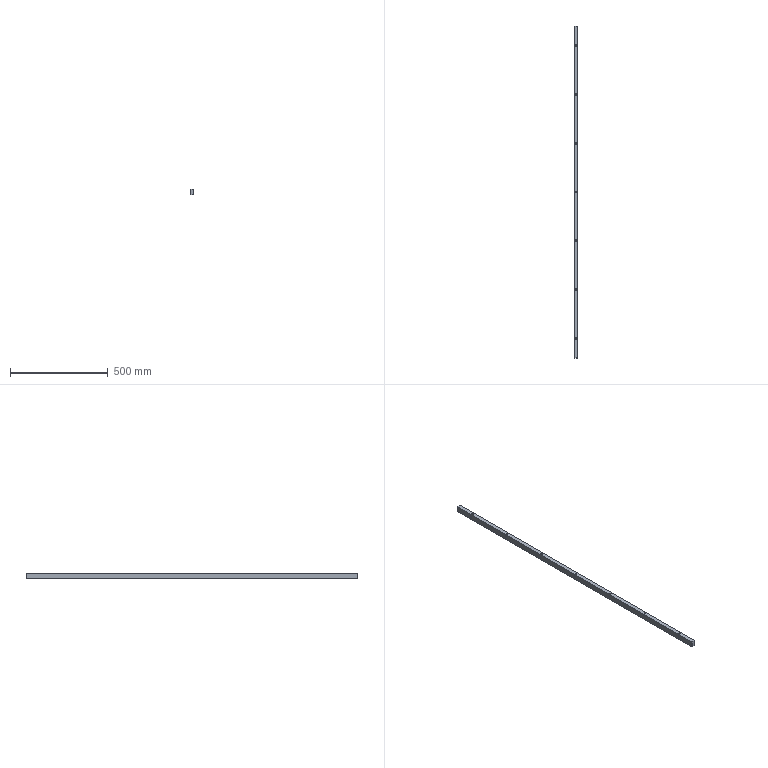Part | SolidWorks | features Chamfer 1, Extrusion 1, HoleWzd 1 | 1 solid | 45 faces | box 18 x 1700 x 30 mm | volume 889358 mm3 | cylinder 28 | plane 17 | commonest cylinder face diameters 9 x14 15 x14
STEP:
#1=CARTESIAN_POINT('',(16.5,1600.,-11.));
#2=VERTEX_POINT('',#1);
#3=CARTESIAN_POINT('',(1.5,1600.,-11.));
#4=VERTEX_POINT('',#3);
#5=CARTESIAN_POINT('',(9.,1600.,-11.));
#6=DIRECTION('',(0.,0.,-1.));
#7=DIRECTION('',(-1.,0.,0.));
#8=AXIS2_PLACEMENT_3D('',#5,#6,#7);
#9=CIRCLE('',#8,7.5);
#10=EDGE_CURVE('',#2,#4,#9,.T.);
#11=ORIENTED_EDGE('',*,*,#10,.F.);
#12=CARTESIAN_POINT('',(16.5,1600.,-30.));
#13=VERTEX_POINT('',#12);
#14=CARTESIAN_POINT('',(16.5,1600.,-30.));
#15=DIRECTION('',(0.,0.,-1.));
#16=VECTOR('',#15,1000.);
#17=LINE('',#14,#16);
#18=EDGE_CURVE('',#2,#13,#17,.T.);
#19=ORIENTED_EDGE('',*,*,#18,.T.);
#20=CARTESIAN_POINT('',(1.5,1600.,-30.));
#21=VERTEX_POINT('',#20);
#22=CARTESIAN_POINT('',(9.,1600.,-30.));
#23=DIRECTION('',(0.,0.,-1.));
#24=DIRECTION('',(-1.,0.,0.));
#25=AXIS2_PLACEMENT_3D('',#22,#23,#24);
#26=CIRCLE('',#25,7.5);
#27=EDGE_CURVE('',#13,#21,#26,.T.);
#28=ORIENTED_EDGE('',*,*,#27,.T.);
#29=CARTESIAN_POINT('',(1.5,1600.,-30.));
#30=DIRECTION('',(0.,0.,-1.));
#31=VECTOR('',#30,1000.);
#32=LINE('',#29,#31);
#33=EDGE_CURVE('',#4,#21,#32,.T.);
#34=ORIENTED_EDGE('',*,*,#33,.F.);
#35=EDGE_LOOP('',(#11,#19,#28,#34));
#36=FACE_OUTER_BOUND('',#35,.T.);
#37=CARTESIAN_POINT('',(9.,1600.,-30.));
#38=DIRECTION('',(0.,0.,-1.));
#39=DIRECTION('',(-1.,0.,0.));
#40=AXIS2_PLACEMENT_3D('',#37,#38,#39);
#41=CYLINDRICAL_SURFACE('',#40,7.5);
#42=ADVANCED_FACE('',(#36),#41,.F.);
#43=CARTESIAN_POINT('',(13.5,1600.,0.));
#44=VERTEX_POINT('',#43);
#45=CARTESIAN_POINT('',(4.5,1600.,0.));
#46=VERTEX_POINT('',#45);
#47=CARTESIAN_POINT('',(9.,1600.,0.));
#48=DIRECTION('',(0.,0.,-1.));
#49=DIRECTION('',(-1.,0.,0.));
#50=AXIS2_PLACEMENT_3D('',#47,#48,#49);
#51=CIRCLE('',#50,4.5);
#52=EDGE_CURVE('',#44,#46,#51,.T.);
#53=ORIENTED_EDGE('',*,*,#52,.F.);
#54=CARTESIAN_POINT('',(13.5,1600.,-11.));
#55=VERTEX_POINT('',#54);
#56=CARTESIAN_POINT('',(13.5,1600.,-30.));
#57=DIRECTION('',(0.,0.,-1.));
#58=VECTOR('',#57,1000.);
#59=LINE('',#56,#58);
#60=EDGE_CURVE('',#44,#55,#59,.T.);
#61=ORIENTED_EDGE('',*,*,#60,.T.);
#62=CARTESIAN_POINT('',(4.5,1600.,-11.));
#63=VERTEX_POINT('',#62);
#64=CARTESIAN_POINT('',(9.,1600.,-11.));
#65=DIRECTION('',(0.,0.,-1.));
#66=DIRECTION('',(-1.,0.,0.));
#67=AXIS2_PLACEMENT_3D('',#64,#65,#66);
#68=CIRCLE('',#67,4.5);
#69=EDGE_CURVE('',#55,#63,#68,.T.);
#70=ORIENTED_EDGE('',*,*,#69,.T.);
#71=CARTESIAN_POINT('',(4.5,1600.,-30.));
#72=DIRECTION('',(0.,0.,-1.));
#73=VECTOR('',#72,1000.);
#74=LINE('',#71,#73);
#75=EDGE_CURVE('',#46,#63,#74,.T.);
#76=ORIENTED_EDGE('',*,*,#75,.F.);
#77=EDGE_LOOP('',(#53,#61,#70,#76));
#78=FACE_OUTER_BOUND('',#77,.T.);
#79=CARTESIAN_POINT('',(9.,1600.,-30.));
#80=DIRECTION('',(0.,0.,-1.));
#81=DIRECTION('',(-1.,0.,0.));
#82=AXIS2_PLACEMENT_3D('',#79,#80,#81);
#83=CYLINDRICAL_SURFACE('',#82,4.5);
#84=ADVANCED_FACE('',(#78),#83,.F.);
#85=CARTESIAN_POINT('',(16.5,1350.,-11.));
#86=VERTEX_POINT('',#85);
#87=CARTESIAN_POINT('',(1.5,1350.,-11.));
#88=VERTEX_POINT('',#87);
#89=CARTESIAN_POINT('',(9.,1350.,-11.));
#90=DIRECTION('',(0.,0.,-1.));
#91=DIRECTION('',(-1.,0.,0.));
#92=AXIS2_PLACEMENT_3D('',#89,#90,#91);
#93=CIRCLE('',#92,7.5);
#94=EDGE_CURVE('',#86,#88,#93,.T.);
#95=ORIENTED_EDGE('',*,*,#94,.F.);
#96=CARTESIAN_POINT('',(16.5,1350.,-30.));
#97=VERTEX_POINT('',#96);
#98=CARTESIAN_POINT('',(16.5,1350.,-30.));
#99=DIRECTION('',(0.,0.,-1.));
#100=VECTOR('',#99,1000.);
#101=LINE('',#98,#100);
#102=EDGE_CURVE('',#86,#97,#101,.T.);
#103=ORIENTED_EDGE('',*,*,#102,.T.);
#104=CARTESIAN_POINT('',(1.5,1350.,-30.));
#105=VERTEX_POINT('',#104);
#106=CARTESIAN_POINT('',(9.,1350.,-30.));
#107=DIRECTION('',(0.,0.,-1.));
#108=DIRECTION('',(-1.,0.,0.));
#109=AXIS2_PLACEMENT_3D('',#106,#107,#108);
#110=CIRCLE('',#109,7.5);
#111=EDGE_CURVE('',#97,#105,#110,.T.);
#112=ORIENTED_EDGE('',*,*,#111,.T.);
#113=CARTESIAN_POINT('',(1.5,1350.,-30.));
#114=DIRECTION('',(0.,0.,-1.));
#115=VECTOR('',#114,1000.);
#116=LINE('',#113,#115);
#117=EDGE_CURVE('',#88,#105,#116,.T.);
#118=ORIENTED_EDGE('',*,*,#117,.F.);
#119=EDGE_LOOP('',(#95,#103,#112,#118));
#120=FACE_OUTER_BOUND('',#119,.T.);
#121=CARTESIAN_POINT('',(9.,1350.,-30.));
#122=DIRECTION('',(0.,0.,-1.));
#123=DIRECTION('',(-1.,0.,0.));
#124=AXIS2_PLACEMENT_3D('',#121,#122,#123);
#125=CYLINDRICAL_SURFACE('',#124,7.5);
#126=ADVANCED_FACE('',(#120),#125,.F.);
#127=CARTESIAN_POINT('',(13.5,1350.,0.));
#128=VERTEX_POINT('',#127);
#129=CARTESIAN_POINT('',(4.5,1350.,0.));
#130=VERTEX_POINT('',#129);
#131=CARTESIAN_POINT('',(9.,1350.,0.));
#132=DIRECTION('',(0.,0.,-1.));
#133=DIRECTION('',(-1.,0.,0.));
#134=AXIS2_PLACEMENT_3D('',#131,#132,#133);
#135=CIRCLE('',#134,4.5);
#136=EDGE_CURVE('',#128,#130,#135,.T.);
#137=ORIENTED_EDGE('',*,*,#136,.F.);
#138=CARTESIAN_POINT('',(13.5,1350.,-11.));
#139=VERTEX_POINT('',#138);
#140=CARTESIAN_POINT('',(13.5,1350.,-30.));
#141=DIRECTION('',(0.,0.,-1.));
#142=VECTOR('',#141,1000.);
#143=LINE('',#140,#142);
#144=EDGE_CURVE('',#128,#139,#143,.T.);
#145=ORIENTED_EDGE('',*,*,#144,.T.);
#146=CARTESIAN_POINT('',(4.5,1350.,-11.));
#147=VERTEX_POINT('',#146);
#148=CARTESIAN_POINT('',(9.,1350.,-11.));
#149=DIRECTION('',(0.,0.,-1.));
#150=DIRECTION('',(-1.,0.,0.));
#151=AXIS2_PLACEMENT_3D('',#148,#149,#150);
#152=CIRCLE('',#151,4.5);
#153=EDGE_CURVE('',#139,#147,#152,.T.);
#154=ORIENTED_EDGE('',*,*,#153,.T.);
#155=CARTESIAN_POINT('',(4.5,1350.,-30.));
#156=DIRECTION('',(0.,0.,-1.));
#157=VECTOR('',#156,1000.);
#158=LINE('',#155,#157);
#159=EDGE_CURVE('',#130,#147,#158,.T.);
#160=ORIENTED_EDGE('',*,*,#159,.F.);
#161=EDGE_LOOP('',(#137,#145,#154,#160));
#162=FACE_OUTER_BOUND('',#161,.T.);
#163=CARTESIAN_POINT('',(9.,1350.,-30.));
#164=DIRECTION('',(0.,0.,-1.));
#165=DIRECTION('',(-1.,0.,0.));
#166=AXIS2_PLACEMENT_3D('',#163,#164,#165);
#167=CYLINDRICAL_SURFACE('',#166,4.5);
#168=ADVANCED_FACE('',(#162),#167,.F.);
#169=CARTESIAN_POINT('',(16.5,1100.,-11.));
#170=VERTEX_POINT('',#169);
#171=CARTESIAN_POINT('',(1.5,1100.,-11.));
#172=VERTEX_POINT('',#171);
#173=CARTESIAN_POINT('',(9.,1100.,-11.));
#174=DIRECTION('',(0.,0.,-1.));
#175=DIRECTION('',(-1.,0.,0.));
#176=AXIS2_PLACEMENT_3D('',#173,#174,#175);
#177=CIRCLE('',#176,7.5);
#178=EDGE_CURVE('',#170,#172,#177,.T.);
#179=ORIENTED_EDGE('',*,*,#178,.F.);
#180=CARTESIAN_POINT('',(16.5,1100.,-30.));
#181=VERTEX_POINT('',#180);
#182=CARTESIAN_POINT('',(16.5,1100.,-30.));
#183=DIRECTION('',(0.,0.,-1.));
#184=VECTOR('',#183,1000.);
#185=LINE('',#182,#184);
#186=EDGE_CURVE('',#170,#181,#185,.T.);
#187=ORIENTED_EDGE('',*,*,#186,.T.);
#188=CARTESIAN_POINT('',(1.5,1100.,-30.));
#189=VERTEX_POINT('',#188);
#190=CARTESIAN_POINT('',(9.,1100.,-30.));
#191=DIRECTION('',(0.,0.,-1.));
#192=DIRECTION('',(-1.,0.,0.));
#193=AXIS2_PLACEMENT_3D('',#190,#191,#192);
#194=CIRCLE('',#193,7.5);
#195=EDGE_CURVE('',#181,#189,#194,.T.);
#196=ORIENTED_EDGE('',*,*,#195,.T.);
#197=CARTESIAN_POINT('',(1.5,1100.,-30.));
#198=DIRECTION('',(0.,0.,-1.));
#199=VECTOR('',#198,1000.);
#200=LINE('',#197,#199);
#201=EDGE_CURVE('',#172,#189,#200,.T.);
#202=ORIENTED_EDGE('',*,*,#201,.F.);
#203=EDGE_LOOP('',(#179,#187,#196,#202));
#204=FACE_OUTER_BOUND('',#203,.T.);
#205=CARTESIAN_POINT('',(9.,1100.,-30.));
#206=DIRECTION('',(0.,0.,-1.));
#207=DIRECTION('',(-1.,0.,0.));
#208=AXIS2_PLACEMENT_3D('',#205,#206,#207);
#209=CYLINDRICAL_SURFACE('',#208,7.5);
#210=ADVANCED_FACE('',(#204),#209,.F.);
#211=CARTESIAN_POINT('',(13.5,1100.,0.));
#212=VERTEX_POINT('',#211);
#213=CARTESIAN_POINT('',(4.5,1100.,0.));
#214=VERTEX_POINT('',#213);
#215=CARTESIAN_POINT('',(9.,1100.,0.));
#216=DIRECTION('',(0.,0.,-1.));
#217=DIRECTION('',(-1.,0.,0.));
#218=AXIS2_PLACEMENT_3D('',#215,#216,#217);
#219=CIRCLE('',#218,4.5);
#220=EDGE_CURVE('',#212,#214,#219,.T.);
#221=ORIENTED_EDGE('',*,*,#220,.F.);
#222=CARTESIAN_POINT('',(13.5,1100.,-11.));
#223=VERTEX_POINT('',#222);
#224=CARTESIAN_POINT('',(13.5,1100.,-30.));
#225=DIRECTION('',(0.,0.,-1.));
#226=VECTOR('',#225,1000.);
#227=LINE('',#224,#226);
#228=EDGE_CURVE('',#212,#223,#227,.T.);
#229=ORIENTED_EDGE('',*,*,#228,.T.);
#230=CARTESIAN_POINT('',(4.5,1100.,-11.));
#231=VERTEX_POINT('',#230);
#232=CARTESIAN_POINT('',(9.,1100.,-11.));
#233=DIRECTION('',(0.,0.,-1.));
#234=DIRECTION('',(-1.,0.,0.));
#235=AXIS2_PLACEMENT_3D('',#232,#233,#234);
#236=CIRCLE('',#235,4.5);
#237=EDGE_CURVE('',#223,#231,#236,.T.);
#238=ORIENTED_EDGE('',*,*,#237,.T.);
#239=CARTESIAN_POINT('',(4.5,1100.,-30.));
#240=DIRECTION('',(0.,0.,-1.));
#241=VECTOR('',#240,1000.);
#242=LINE('',#239,#241);
#243=EDGE_CURVE('',#214,#231,#242,.T.);
#244=ORIENTED_EDGE('',*,*,#243,.F.);
#245=EDGE_LOOP('',(#221,#229,#238,#244));
#246=FACE_OUTER_BOUND('',#245,.T.);
#247=CARTESIAN_POINT('',(9.,1100.,-30.));
#248=DIRECTION('',(0.,0.,-1.));
#249=DIRECTION('',(-1.,0.,0.));
#250=AXIS2_PLACEMENT_3D('',#247,#248,#249);
#251=CYLINDRICAL_SURFACE('',#250,4.5);
#252=ADVANCED_FACE('',(#246),#251,.F.);
#253=CARTESIAN_POINT('',(16.5,600.,-11.));
#254=VERTEX_POINT('',#253);
#255=CARTESIAN_POINT('',(1.5,600.,-11.));
#256=VERTEX_POINT('',#255);
#257=CARTESIAN_POINT('',(9.,600.,-11.));
#258=DIRECTION('',(0.,0.,-1.));
#259=DIRECTION('',(-1.,0.,0.));
#260=AXIS2_PLACEMENT_3D('',#257,#258,#259);
#261=CIRCLE('',#260,7.5);
#262=EDGE_CURVE('',#254,#256,#261,.T.);
#263=ORIENTED_EDGE('',*,*,#262,.F.);
#264=CARTESIAN_POINT('',(16.5,600.,-30.));
#265=VERTEX_POINT('',#264);
#266=CARTESIAN_POINT('',(16.5,600.,-30.));
#267=DIRECTION('',(0.,0.,-1.));
#268=VECTOR('',#267,1000.);
#269=LINE('',#266,#268);
#270=EDGE_CURVE('',#254,#265,#269,.T.);
#271=ORIENTED_EDGE('',*,*,#270,.T.);
#272=CARTESIAN_POINT('',(1.5,600.,-30.));
#273=VERTEX_POINT('',#272);
#274=CARTESIAN_POINT('',(9.,600.,-30.));
#275=DIRECTION('',(0.,0.,-1.));
#276=DIRECTION('',(-1.,0.,0.));
#277=AXIS2_PLACEMENT_3D('',#274,#275,#276);
#278=CIRCLE('',#277,7.5);
#279=EDGE_CURVE('',#265,#273,#278,.T.);
#280=ORIENTED_EDGE('',*,*,#279,.T.);
#281=CARTESIAN_POINT('',(1.5,600.,-30.));
#282=DIRECTION('',(0.,0.,-1.));
#283=VECTOR('',#282,1000.);
#284=LINE('',#281,#283);
#285=EDGE_CURVE('',#256,#273,#284,.T.);
#286=ORIENTED_EDGE('',*,*,#285,.F.);
#287=EDGE_LOOP('',(#263,#271,#280,#286));
#288=FACE_OUTER_BOUND('',#287,.T.);
#289=CARTESIAN_POINT('',(9.,600.,-30.));
#290=DIRECTION('',(0.,0.,-1.));
#291=DIRECTION('',(-1.,0.,0.));
#292=AXIS2_PLACEMENT_3D('',#289,#290,#291);
#293=CYLINDRICAL_SURFACE('',#292,7.5);
#294=ADVANCED_FACE('',(#288),#293,.F.);
#295=CARTESIAN_POINT('',(13.5,600.,0.));
#296=VERTEX_POINT('',#295);
#297=CARTESIAN_POINT('',(4.5,600.,0.));
#298=VERTEX_POINT('',#297);
#299=CARTESIAN_POINT('',(9.,600.,0.));
#300=DIRECTION('',(0.,0.,-1.));
#301=DIRECTION('',(-1.,0.,0.));
#302=AXIS2_PLACEMENT_3D('',#299,#300,#301);
#303=CIRCLE('',#302,4.5);
#304=EDGE_CURVE('',#296,#298,#303,.T.);
#305=ORIENTED_EDGE('',*,*,#304,.F.);
#306=CARTESIAN_POINT('',(13.5,600.,-11.));
#307=VERTEX_POINT('',#306);
#308=CARTESIAN_POINT('',(13.5,600.,-30.));
#309=DIRECTION('',(0.,0.,-1.));
#310=VECTOR('',#309,1000.);
#311=LINE('',#308,#310);
#312=EDGE_CURVE('',#296,#307,#311,.T.);
#313=ORIENTED_EDGE('',*,*,#312,.T.);
#314=CARTESIAN_POINT('',(4.5,600.,-11.));
#315=VERTEX_POINT('',#314);
#316=CARTESIAN_POINT('',(9.,600.,-11.));
#317=DIRECTION('',(0.,0.,-1.));
#318=DIRECTION('',(-1.,0.,0.));
#319=AXIS2_PLACEMENT_3D('',#316,#317,#318);
#320=CIRCLE('',#319,4.5);
#321=EDGE_CURVE('',#307,#315,#320,.T.);
#322=ORIENTED_EDGE('',*,*,#321,.T.);
#323=CARTESIAN_POINT('',(4.5,600.,-30.));
#324=DIRECTION('',(0.,0.,-1.));
#325=VECTOR('',#324,1000.);
#326=LINE('',#323,#325);
#327=EDGE_CURVE('',#298,#315,#326,.T.);
#328=ORIENTED_EDGE('',*,*,#327,.F.);
#329=EDGE_LOOP('',(#305,#313,#322,#328));
#330=FACE_OUTER_BOUND('',#329,.T.);
#331=CARTESIAN_POINT('',(9.,600.,-30.));
#332=DIRECTION('',(0.,0.,-1.));
#333=DIRECTION('',(-1.,0.,0.));
#334=AXIS2_PLACEMENT_3D('',#331,#332,#333);
#335=CYLINDRICAL_SURFACE('',#334,4.5);
#336=ADVANCED_FACE('',(#330),#335,.F.);
#337=CARTESIAN_POINT('',(16.5,350.,-11.));
#338=VERTEX_POINT('',#337);
#339=CARTESIAN_POINT('',(1.5,350.,-11.));
#340=VERTEX_POINT('',#339);
#341=CARTESIAN_POINT('',(9.,350.,-11.));
#342=DIRECTION('',(0.,0.,-1.));
#343=DIRECTION('',(-1.,0.,0.));
#344=AXIS2_PLACEMENT_3D('',#341,#342,#343);
#345=CIRCLE('',#344,7.5);
#346=EDGE_CURVE('',#338,#340,#345,.T.);
#347=ORIENTED_EDGE('',*,*,#346,.F.);
#348=CARTESIAN_POINT('',(16.5,350.,-30.));
#349=VERTEX_POINT('',#348);
#350=CARTESIAN_POINT('',(16.5,350.,-30.));
#351=DIRECTION('',(0.,0.,-1.));
#352=VECTOR('',#351,1000.);
#353=LINE('',#350,#352);
#354=EDGE_CURVE('',#338,#349,#353,.T.);
#355=ORIENTED_EDGE('',*,*,#354,.T.);
#356=CARTESIAN_POINT('',(1.5,350.,-30.));
#357=VERTEX_POINT('',#356);
#358=CARTESIAN_POINT('',(9.,350.,-30.));
#359=DIRECTION('',(0.,0.,-1.));
#360=DIRECTION('',(-1.,0.,0.));
#361=AXIS2_PLACEMENT_3D('',#358,#359,#360);
#362=CIRCLE('',#361,7.5);
#363=EDGE_CURVE('',#349,#357,#362,.T.);
#364=ORIENTED_EDGE('',*,*,#363,.T.);
#365=CARTESIAN_POINT('',(1.5,350.,-30.));
#366=DIRECTION('',(0.,0.,-1.));
#367=VECTOR('',#366,1000.);
#368=LINE('',#365,#367);
#369=EDGE_CURVE('',#340,#357,#368,.T.);
#370=ORIENTED_EDGE('',*,*,#369,.F.);
#371=EDGE_LOOP('',(#347,#355,#364,#370));
#372=FACE_OUTER_BOUND('',#371,.T.);
#373=CARTESIAN_POINT('',(9.,350.,-30.));
#374=DIRECTION('',(0.,0.,-1.));
#375=DIRECTION('',(-1.,0.,0.));
#376=AXIS2_PLACEMENT_3D('',#373,#374,#375);
#377=CYLINDRICAL_SURFACE('',#376,7.5);
#378=ADVANCED_FACE('',(#372),#377,.F.);
#379=CARTESIAN_POINT('',(13.5,350.,0.));
#380=VERTEX_POINT('',#379);
#381=CARTESIAN_POINT('',(4.5,350.,0.));
#382=VERTEX_POINT('',#381);
#383=CARTESIAN_POINT('',(9.,350.,0.));
#384=DIRECTION('',(0.,0.,-1.));
#385=DIRECTION('',(-1.,0.,0.));
#386=AXIS2_PLACEMENT_3D('',#383,#384,#385);
#387=CIRCLE('',#386,4.5);
#388=EDGE_CURVE('',#380,#382,#387,.T.);
#389=ORIENTED_EDGE('',*,*,#388,.F.);
#390=CARTESIAN_POINT('',(13.5,350.,-11.));
#391=VERTEX_POINT('',#390);
#392=CARTESIAN_POINT('',(13.5,350.,-30.));
#393=DIRECTION('',(0.,0.,-1.));
#394=VECTOR('',#393,1000.);
#395=LINE('',#392,#394);
#396=EDGE_CURVE('',#380,#391,#395,.T.);
#397=ORIENTED_EDGE('',*,*,#396,.T.);
#398=CARTESIAN_POINT('',(4.5,350.,-11.));
#399=VERTEX_POINT('',#398);
#400=CARTESIAN_POINT('',(9.,350.,-11.));
#401=DIRECTION('',(0.,0.,-1.));
#402=DIRECTION('',(-1.,0.,0.));
#403=AXIS2_PLACEMENT_3D('',#400,#401,#402);
#404=CIRCLE('',#403,4.5);
#405=EDGE_CURVE('',#391,#399,#404,.T.);
#406=ORIENTED_EDGE('',*,*,#405,.T.);
#407=CARTESIAN_POINT('',(4.5,350.,-30.));
#408=DIRECTION('',(0.,0.,-1.));
#409=VECTOR('',#408,1000.);
#410=LINE('',#407,#409);
#411=EDGE_CURVE('',#382,#399,#410,.T.);
#412=ORIENTED_EDGE('',*,*,#411,.F.);
#413=EDGE_LOOP('',(#389,#397,#406,#412));
#414=FACE_OUTER_BOUND('',#413,.T.);
#415=CARTESIAN_POINT('',(9.,350.,-30.));
#416=DIRECTION('',(0.,0.,-1.));
#417=DIRECTION('',(-1.,0.,0.));
#418=AXIS2_PLACEMENT_3D('',#415,#416,#417);
#419=CYLINDRICAL_SURFACE('',#418,4.5);
#420=ADVANCED_FACE('',(#414),#419,.F.);
#421=CARTESIAN_POINT('',(16.5,100.,-11.));
#422=VERTEX_POINT('',#421);
#423=CARTESIAN_POINT('',(1.5,100.,-11.));
#424=VERTEX_POINT('',#423);
#425=CARTESIAN_POINT('',(9.,100.,-11.));
#426=DIRECTION('',(0.,0.,-1.));
#427=DIRECTION('',(-1.,0.,0.));
#428=AXIS2_PLACEMENT_3D('',#425,#426,#427);
#429=CIRCLE('',#428,7.5);
#430=EDGE_CURVE('',#422,#424,#429,.T.);
#431=ORIENTED_EDGE('',*,*,#430,.F.);
#432=CARTESIAN_POINT('',(16.5,100.,-30.));
#433=VERTEX_POINT('',#432);
#434=CARTESIAN_POINT('',(16.5,100.,-30.));
#435=DIRECTION('',(0.,0.,-1.));
#436=VECTOR('',#435,1000.);
#437=LINE('',#434,#436);
#438=EDGE_CURVE('',#422,#433,#437,.T.);
#439=ORIENTED_EDGE('',*,*,#438,.T.);
#440=CARTESIAN_POINT('',(1.5,100.,-30.));
#441=VERTEX_POINT('',#440);
#442=CARTESIAN_POINT('',(9.,100.,-30.));
#443=DIRECTION('',(0.,0.,-1.));
#444=DIRECTION('',(-1.,0.,0.));
#445=AXIS2_PLACEMENT_3D('',#442,#443,#444);
#446=CIRCLE('',#445,7.5);
#447=EDGE_CURVE('',#433,#441,#446,.T.);
#448=ORIENTED_EDGE('',*,*,#447,.T.);
#449=CARTESIAN_POINT('',(1.5,100.,-30.));
#450=DIRECTION('',(0.,0.,-1.));
#451=VECTOR('',#450,1000.);
#452=LINE('',#449,#451);
#453=EDGE_CURVE('',#424,#441,#452,.T.);
#454=ORIENTED_EDGE('',*,*,#453,.F.);
#455=EDGE_LOOP('',(#431,#439,#448,#454));
#456=FACE_OUTER_BOUND('',#455,.T.);
#457=CARTESIAN_POINT('',(9.,100.,-30.));
#458=DIRECTION('',(0.,0.,-1.));
#459=DIRECTION('',(-1.,0.,0.));
#460=AXIS2_PLACEMENT_3D('',#457,#458,#459);
#461=CYLINDRICAL_SURFACE('',#460,7.5);
#462=ADVANCED_FACE('',(#456),#461,.F.);
#463=CARTESIAN_POINT('',(13.5,100.,0.));
#464=VERTEX_POINT('',#463);
#465=CARTESIAN_POINT('',(4.5,100.,0.));
#466=VERTEX_POINT('',#465);
#467=CARTESIAN_POINT('',(9.,100.,0.));
#468=DIRECTION('',(0.,0.,-1.));
#469=DIRECTION('',(-1.,0.,0.));
#470=AXIS2_PLACEMENT_3D('',#467,#468,#469);
#471=CIRCLE('',#470,4.5);
#472=EDGE_CURVE('',#464,#466,#471,.T.);
#473=ORIENTED_EDGE('',*,*,#472,.F.);
#474=CARTESIAN_POINT('',(13.5,100.,-11.));
#475=VERTEX_POINT('',#474);
#476=CARTESIAN_POINT('',(13.5,100.,-30.));
#477=DIRECTION('',(0.,0.,-1.));
#478=VECTOR('',#477,1000.);
#479=LINE('',#476,#478);
#480=EDGE_CURVE('',#464,#475,#479,.T.);
#481=ORIENTED_EDGE('',*,*,#480,.T.);
#482=CARTESIAN_POINT('',(4.5,100.,-11.));
#483=VERTEX_POINT('',#482);
#484=CARTESIAN_POINT('',(9.,100.,-11.));
#485=DIRECTION('',(0.,0.,-1.));
#486=DIRECTION('',(-1.,0.,0.));
#487=AXIS2_PLACEMENT_3D('',#484,#485,#486);
#488=CIRCLE('',#487,4.5);
#489=EDGE_CURVE('',#475,#483,#488,.T.);
#490=ORIENTED_EDGE('',*,*,#489,.T.);
#491=CARTESIAN_POINT('',(4.5,100.,-30.));
#492=DIRECTION('',(0.,0.,-1.));
#493=VECTOR('',#492,1000.);
#494=LINE('',#491,#493);
#495=EDGE_CURVE('',#466,#483,#494,.T.);
#496=ORIENTED_EDGE('',*,*,#495,.F.);
#497=EDGE_LOOP('',(#473,#481,#490,#496));
#498=FACE_OUTER_BOUND('',#497,.T.);
#499=CARTESIAN_POINT('',(9.,100.,-30.));
#500=DIRECTION('',(0.,0.,-1.));
#501=DIRECTION('',(-1.,0.,0.));
#502=AXIS2_PLACEMENT_3D('',#499,#500,#501);
#503=CYLINDRICAL_SURFACE('',#502,4.5);
#504=ADVANCED_FACE('',(#498),#503,.F.);
#505=CARTESIAN_POINT('',(16.5,850.,-11.));
#506=VERTEX_POINT('',#505);
#507=CARTESIAN_POINT('',(1.5,850.,-11.));
#508=VERTEX_POINT('',#507);
#509=CARTESIAN_POINT('',(9.,850.,-11.));
#510=DIRECTION('',(0.,0.,-1.));
#511=DIRECTION('',(-1.,0.,0.));
#512=AXIS2_PLACEMENT_3D('',#509,#510,#511);
#513=CIRCLE('',#512,7.5);
#514=EDGE_CURVE('',#506,#508,#513,.T.);
#515=ORIENTED_EDGE('',*,*,#514,.F.);
#516=CARTESIAN_POINT('',(16.5,850.,-30.));
#517=VERTEX_POINT('',#516);
#518=CARTESIAN_POINT('',(16.5,850.,-30.));
#519=DIRECTION('',(0.,0.,-1.));
#520=VECTOR('',#519,1000.);
#521=LINE('',#518,#520);
#522=EDGE_CURVE('',#506,#517,#521,.T.);
#523=ORIENTED_EDGE('',*,*,#522,.T.);
#524=CARTESIAN_POINT('',(1.5,850.,-30.));
#525=VERTEX_POINT('',#524);
#526=CARTESIAN_POINT('',(9.,850.,-30.));
#527=DIRECTION('',(0.,0.,-1.));
#528=DIRECTION('',(-1.,0.,0.));
#529=AXIS2_PLACEMENT_3D('',#526,#527,#528);
#530=CIRCLE('',#529,7.5);
#531=EDGE_CURVE('',#517,#525,#530,.T.);
#532=ORIENTED_EDGE('',*,*,#531,.T.);
#533=CARTESIAN_POINT('',(1.5,850.,-30.));
#534=DIRECTION('',(0.,0.,-1.));
#535=VECTOR('',#534,1000.);
#536=LINE('',#533,#535);
#537=EDGE_CURVE('',#508,#525,#536,.T.);
#538=ORIENTED_EDGE('',*,*,#537,.F.);
#539=EDGE_LOOP('',(#515,#523,#532,#538));
#540=FACE_OUTER_BOUND('',#539,.T.);
#541=CARTESIAN_POINT('',(9.,850.,-30.));
#542=DIRECTION('',(0.,0.,-1.));
#543=DIRECTION('',(-1.,0.,0.));
#544=AXIS2_PLACEMENT_3D('',#541,#542,#543);
#545=CYLINDRICAL_SURFACE('',#544,7.5);
#546=ADVANCED_FACE('',(#540),#545,.F.);
#547=CARTESIAN_POINT('',(13.5,850.,0.));
#548=VERTEX_POINT('',#547);
#549=CARTESIAN_POINT('',(4.5,850.,0.));
#550=VERTEX_POINT('',#549);
#551=CARTESIAN_POINT('',(9.,850.,0.));
#552=DIRECTION('',(0.,0.,-1.));
#553=DIRECTION('',(-1.,0.,0.));
#554=AXIS2_PLACEMENT_3D('',#551,#552,#553);
#555=CIRCLE('',#554,4.5);
#556=EDGE_CURVE('',#548,#550,#555,.T.);
#557=ORIENTED_EDGE('',*,*,#556,.F.);
#558=CARTESIAN_POINT('',(13.5,850.,-11.));
#559=VERTEX_POINT('',#558);
#560=CARTESIAN_POINT('',(13.5,850.,-30.));
#561=DIRECTION('',(0.,0.,-1.));
#562=VECTOR('',#561,1000.);
#563=LINE('',#560,#562);
#564=EDGE_CURVE('',#548,#559,#563,.T.);
#565=ORIENTED_EDGE('',*,*,#564,.T.);
#566=CARTESIAN_POINT('',(4.5,850.,-11.));
#567=VERTEX_POINT('',#566);
#568=CARTESIAN_POINT('',(9.,850.,-11.));
#569=DIRECTION('',(0.,0.,-1.));
#570=DIRECTION('',(-1.,0.,0.));
#571=AXIS2_PLACEMENT_3D('',#568,#569,#570);
#572=CIRCLE('',#571,4.5);
#573=EDGE_CURVE('',#559,#567,#572,.T.);
#574=ORIENTED_EDGE('',*,*,#573,.T.);
#575=CARTESIAN_POINT('',(4.5,850.,-30.));
#576=DIRECTION('',(0.,0.,-1.));
#577=VECTOR('',#576,1000.);
#578=LINE('',#575,#577);
#579=EDGE_CURVE('',#550,#567,#578,.T.);
#580=ORIENTED_EDGE('',*,*,#579,.F.);
#581=EDGE_LOOP('',(#557,#565,#574,#580));
#582=FACE_OUTER_BOUND('',#581,.T.);
#583=CARTESIAN_POINT('',(9.,850.,-30.));
#584=DIRECTION('',(0.,0.,-1.));
#585=DIRECTION('',(-1.,0.,0.));
#586=AXIS2_PLACEMENT_3D('',#583,#584,#585);
#587=CYLINDRICAL_SURFACE('',#586,4.5);
#588=ADVANCED_FACE('',(#582),#587,.F.);
#589=CARTESIAN_POINT('',(9.,1600.,-30.));
#590=DIRECTION('',(0.,0.,-1.));
#591=DIRECTION('',(-1.,0.,0.));
#592=AXIS2_PLACEMENT_3D('',#589,#590,#591);
#593=CIRCLE('',#592,7.5);
#594=EDGE_CURVE('',#21,#13,#593,.T.);
#595=ORIENTED_EDGE('',*,*,#594,.F.);
#596=ORIENTED_EDGE('',*,*,#27,.F.);
#597=EDGE_LOOP('',(#595,#596));
#598=FACE_BOUND('',#597,.T.);
#599=CARTESIAN_POINT('',(9.,600.,-30.));
#600=DIRECTION('',(0.,0.,-1.));
#601=DIRECTION('',(-1.,0.,0.));
#602=AXIS2_PLACEMENT_3D('',#599,#600,#601);
#603=CIRCLE('',#602,7.5);
#604=EDGE_CURVE('',#273,#265,#603,.T.);
#605=ORIENTED_EDGE('',*,*,#604,.F.);
#606=ORIENTED_EDGE('',*,*,#279,.F.);
#607=EDGE_LOOP('',(#605,#606));
#608=FACE_BOUND('',#607,.T.);
#609=CARTESIAN_POINT('',(9.,100.,-30.));
#610=DIRECTION('',(0.,0.,-1.));
#611=DIRECTION('',(-1.,0.,0.));
#612=AXIS2_PLACEMENT_3D('',#609,#610,#611);
#613=CIRCLE('',#612,7.5);
#614=EDGE_CURVE('',#441,#433,#613,.T.);
#615=ORIENTED_EDGE('',*,*,#614,.F.);
#616=ORIENTED_EDGE('',*,*,#447,.F.);
#617=EDGE_LOOP('',(#615,#616));
#618=FACE_BOUND('',#617,.T.);
#619=CARTESIAN_POINT('',(9.,850.,-30.));
#620=DIRECTION('',(0.,0.,-1.));
#621=DIRECTION('',(-1.,0.,0.));
#622=AXIS2_PLACEMENT_3D('',#619,#620,#621);
#623=CIRCLE('',#622,7.5);
#624=EDGE_CURVE('',#525,#517,#623,.T.);
#625=ORIENTED_EDGE('',*,*,#624,.F.);
#626=ORIENTED_EDGE('',*,*,#531,.F.);
#627=EDGE_LOOP('',(#625,#626));
#628=FACE_BOUND('',#627,.T.);
#629=CARTESIAN_POINT('',(16.,0.,-30.));
#630=VERTEX_POINT('',#629);
#631=CARTESIAN_POINT('',(2.,0.,-30.));
#632=VERTEX_POINT('',#631);
#633=CARTESIAN_POINT('',(0.,0.,-30.));
#634=DIRECTION('',(-1.,0.,0.));
#635=VECTOR('',#634,1000.);
#636=LINE('',#633,#635);
#637=EDGE_CURVE('',#630,#632,#636,.T.);
#638=ORIENTED_EDGE('',*,*,#637,.T.);
#639=CARTESIAN_POINT('',(0.,2.,-30.));
#640=VERTEX_POINT('',#639);
#641=CARTESIAN_POINT('',(0.,2.,-30.));
#642=DIRECTION('',(-0.7071,0.7071,0.));
#643=VECTOR('',#642,1000.);
#644=LINE('',#641,#643);
#645=EDGE_CURVE('',#632,#640,#644,.T.);
#646=ORIENTED_EDGE('',*,*,#645,.T.);
#647=CARTESIAN_POINT('',(0.,1698.,-30.));
#648=VERTEX_POINT('',#647);
#649=CARTESIAN_POINT('',(0.,1700.,-30.));
#650=DIRECTION('',(0.,-1.,0.));
#651=VECTOR('',#650,1000.);
#652=LINE('',#649,#651);
#653=EDGE_CURVE('',#648,#640,#652,.T.);
#654=ORIENTED_EDGE('',*,*,#653,.F.);
#655=CARTESIAN_POINT('',(2.,1700.,-30.));
#656=VERTEX_POINT('',#655);
#657=CARTESIAN_POINT('',(2.,1700.,-30.));
#658=DIRECTION('',(0.7071,0.7071,0.));
#659=VECTOR('',#658,1000.);
#660=LINE('',#657,#659);
#661=EDGE_CURVE('',#648,#656,#660,.T.);
#662=ORIENTED_EDGE('',*,*,#661,.T.);
#663=CARTESIAN_POINT('',(16.,1700.,-30.));
#664=VERTEX_POINT('',#663);
#665=CARTESIAN_POINT('',(0.,1700.,-30.));
#666=DIRECTION('',(-1.,0.,0.));
#667=VECTOR('',#666,1000.);
#668=LINE('',#665,#667);
#669=EDGE_CURVE('',#664,#656,#668,.T.);
#670=ORIENTED_EDGE('',*,*,#669,.F.);
#671=CARTESIAN_POINT('',(18.,1698.,-30.));
#672=VERTEX_POINT('',#671);
#673=CARTESIAN_POINT('',(16.,1700.,-30.));
#674=DIRECTION('',(0.7071,-0.7071,0.));
#675=VECTOR('',#674,1000.);
#676=LINE('',#673,#675);
#677=EDGE_CURVE('',#664,#672,#676,.T.);
#678=ORIENTED_EDGE('',*,*,#677,.T.);
#679=CARTESIAN_POINT('',(18.,2.,-30.));
#680=VERTEX_POINT('',#679);
#681=CARTESIAN_POINT('',(18.,1700.,-30.));
#682=DIRECTION('',(0.,-1.,0.));
#683=VECTOR('',#682,1000.);
#684=LINE('',#681,#683);
#685=EDGE_CURVE('',#672,#680,#684,.T.);
#686=ORIENTED_EDGE('',*,*,#685,.T.);
#687=CARTESIAN_POINT('',(18.,2.,-30.));
#688=DIRECTION('',(-0.7071,-0.7071,0.));
#689=VECTOR('',#688,1000.);
#690=LINE('',#687,#689);
#691=EDGE_CURVE('',#680,#630,#690,.T.);
#692=ORIENTED_EDGE('',*,*,#691,.T.);
#693=EDGE_LOOP('',(#638,#646,#654,#662,#670,#678,#686,#692));
#694=FACE_OUTER_BOUND('',#693,.T.);
#695=CARTESIAN_POINT('',(9.,350.,-30.));
#696=DIRECTION('',(0.,0.,-1.));
#697=DIRECTION('',(-1.,0.,0.));
#698=AXIS2_PLACEMENT_3D('',#695,#696,#697);
#699=CIRCLE('',#698,7.5);
#700=EDGE_CURVE('',#357,#349,#699,.T.);
#701=ORIENTED_EDGE('',*,*,#700,.F.);
#702=ORIENTED_EDGE('',*,*,#363,.F.);
#703=EDGE_LOOP('',(#701,#702));
#704=FACE_BOUND('',#703,.T.);
#705=CARTESIAN_POINT('',(9.,1100.,-30.));
#706=DIRECTION('',(0.,0.,-1.));
#707=DIRECTION('',(-1.,0.,0.));
#708=AXIS2_PLACEMENT_3D('',#705,#706,#707);
#709=CIRCLE('',#708,7.5);
#710=EDGE_CURVE('',#189,#181,#709,.T.);
#711=ORIENTED_EDGE('',*,*,#710,.F.);
#712=ORIENTED_EDGE('',*,*,#195,.F.);
#713=EDGE_LOOP('',(#711,#712));
#714=FACE_BOUND('',#713,.T.);
#715=CARTESIAN_POINT('',(9.,1350.,-30.));
#716=DIRECTION('',(0.,0.,-1.));
#717=DIRECTION('',(-1.,0.,0.));
#718=AXIS2_PLACEMENT_3D('',#715,#716,#717);
#719=CIRCLE('',#718,7.5);
#720=EDGE_CURVE('',#105,#97,#719,.T.);
#721=ORIENTED_EDGE('',*,*,#720,.F.);
#722=ORIENTED_EDGE('',*,*,#111,.F.);
#723=EDGE_LOOP('',(#721,#722));
#724=FACE_BOUND('',#723,.T.);
#725=CARTESIAN_POINT('',(0.,1700.,-30.));
#726=DIRECTION('',(0.,0.,1.));
#727=DIRECTION('',(1.,0.,0.));
#728=AXIS2_PLACEMENT_3D('',#725,#726,#727);
#729=PLANE('',#728);
#730=ADVANCED_FACE('',(#598,#608,#618,#628,#694,#704,#714,#724),#729,.F.);
#731=ORIENTED_EDGE('',*,*,#653,.T.);
#732=CARTESIAN_POINT('',(0.,2.,0.));
#733=VERTEX_POINT('',#732);
#734=CARTESIAN_POINT('',(0.,2.,0.));
#735=DIRECTION('',(0.,0.,1.));
#736=VECTOR('',#735,1000.);
#737=LINE('',#734,#736);
#738=EDGE_CURVE('',#640,#733,#737,.T.);
#739=ORIENTED_EDGE('',*,*,#738,.T.);
#740=CARTESIAN_POINT('',(0.,1698.,0.));
#741=VERTEX_POINT('',#740);
#742=CARTESIAN_POINT('',(0.,1700.,0.));
#743=DIRECTION('',(0.,-1.,0.));
#744=VECTOR('',#743,1000.);
#745=LINE('',#742,#744);
#746=EDGE_CURVE('',#741,#733,#745,.T.);
#747=ORIENTED_EDGE('',*,*,#746,.F.);
#748=CARTESIAN_POINT('',(0.,1698.,0.));
#749=DIRECTION('',(0.,0.,-1.));
#750=VECTOR('',#749,1000.);
#751=LINE('',#748,#750);
#752=EDGE_CURVE('',#741,#648,#751,.T.);
#753=ORIENTED_EDGE('',*,*,#752,.T.);
#754=EDGE_LOOP('',(#731,#739,#747,#753));
#755=FACE_OUTER_BOUND('',#754,.T.);
#756=CARTESIAN_POINT('',(0.,1700.,0.));
#757=DIRECTION('',(1.,0.,0.));
#758=DIRECTION('',(0.,0.,-1.));
#759=AXIS2_PLACEMENT_3D('',#756,#757,#758);
#760=PLANE('',#759);
#761=ADVANCED_FACE('',(#755),#760,.F.);
#762=CARTESIAN_POINT('',(9.,1600.,0.));
#763=DIRECTION('',(0.,0.,-1.));
#764=DIRECTION('',(-1.,0.,0.));
#765=AXIS2_PLACEMENT_3D('',#762,#763,#764);
#766=CIRCLE('',#765,4.5);
#767=EDGE_CURVE('',#46,#44,#766,.T.);
#768=ORIENTED_EDGE('',*,*,#767,.T.);
#769=ORIENTED_EDGE('',*,*,#52,.T.);
#770=EDGE_LOOP('',(#768,#769));
#771=FACE_BOUND('',#770,.T.);
#772=CARTESIAN_POINT('',(9.,1350.,0.));
#773=DIRECTION('',(0.,0.,-1.));
#774=DIRECTION('',(-1.,0.,0.));
#775=AXIS2_PLACEMENT_3D('',#772,#773,#774);
#776=CIRCLE('',#775,4.5);
#777=EDGE_CURVE('',#130,#128,#776,.T.);
#778=ORIENTED_EDGE('',*,*,#777,.T.);
#779=ORIENTED_EDGE('',*,*,#136,.T.);
#780=EDGE_LOOP('',(#778,#779));
#781=FACE_BOUND('',#780,.T.);
#782=CARTESIAN_POINT('',(9.,1100.,0.));
#783=DIRECTION('',(0.,0.,-1.));
#784=DIRECTION('',(-1.,0.,0.));
#785=AXIS2_PLACEMENT_3D('',#782,#783,#784);
#786=CIRCLE('',#785,4.5);
#787=EDGE_CURVE('',#214,#212,#786,.T.);
#788=ORIENTED_EDGE('',*,*,#787,.T.);
#789=ORIENTED_EDGE('',*,*,#220,.T.);
#790=EDGE_LOOP('',(#788,#789));
#791=FACE_BOUND('',#790,.T.);
#792=CARTESIAN_POINT('',(9.,600.,0.));
#793=DIRECTION('',(0.,0.,-1.));
#794=DIRECTION('',(-1.,0.,0.));
#795=AXIS2_PLACEMENT_3D('',#792,#793,#794);
#796=CIRCLE('',#795,4.5);
#797=EDGE_CURVE('',#298,#296,#796,.T.);
#798=ORIENTED_EDGE('',*,*,#797,.T.);
#799=ORIENTED_EDGE('',*,*,#304,.T.);
#800=EDGE_LOOP('',(#798,#799));
#801=FACE_BOUND('',#800,.T.);
#802=CARTESIAN_POINT('',(9.,350.,0.));
#803=DIRECTION('',(0.,0.,-1.));
#804=DIRECTION('',(-1.,0.,0.));
#805=AXIS2_PLACEMENT_3D('',#802,#803,#804);
#806=CIRCLE('',#805,4.5);
#807=EDGE_CURVE('',#382,#380,#806,.T.);
#808=ORIENTED_EDGE('',*,*,#807,.T.);
#809=ORIENTED_EDGE('',*,*,#388,.T.);
#810=EDGE_LOOP('',(#808,#809));
#811=FACE_BOUND('',#810,.T.);
#812=CARTESIAN_POINT('',(9.,100.,0.));
#813=DIRECTION('',(0.,0.,-1.));
#814=DIRECTION('',(-1.,0.,0.));
#815=AXIS2_PLACEMENT_3D('',#812,#813,#814);
#816=CIRCLE('',#815,4.5);
#817=EDGE_CURVE('',#466,#464,#816,.T.);
#818=ORIENTED_EDGE('',*,*,#817,.T.);
#819=ORIENTED_EDGE('',*,*,#472,.T.);
#820=EDGE_LOOP('',(#818,#819));
#821=FACE_BOUND('',#820,.T.);
#822=CARTESIAN_POINT('',(9.,850.,0.));
#823=DIRECTION('',(0.,0.,-1.));
#824=DIRECTION('',(-1.,0.,0.));
#825=AXIS2_PLACEMENT_3D('',#822,#823,#824);
#826=CIRCLE('',#825,4.5);
#827=EDGE_CURVE('',#550,#548,#826,.T.);
#828=ORIENTED_EDGE('',*,*,#827,.T.);
#829=ORIENTED_EDGE('',*,*,#556,.T.);
#830=EDGE_LOOP('',(#828,#829));
#831=FACE_BOUND('',#830,.T.);
#832=ORIENTED_EDGE('',*,*,#746,.T.);
#833=CARTESIAN_POINT('',(2.,0.,0.));
#834=VERTEX_POINT('',#833);
#835=CARTESIAN_POINT('',(0.,2.,0.));
#836=DIRECTION('',(0.7071,-0.7071,0.));
#837=VECTOR('',#836,1000.);
#838=LINE('',#835,#837);
#839=EDGE_CURVE('',#733,#834,#838,.T.);
#840=ORIENTED_EDGE('',*,*,#839,.T.);
#841=CARTESIAN_POINT('',(16.,0.,0.));
#842=VERTEX_POINT('',#841);
#843=CARTESIAN_POINT('',(0.,0.,0.));
#844=DIRECTION('',(1.,0.,0.));
#845=VECTOR('',#844,1000.);
#846=LINE('',#843,#845);
#847=EDGE_CURVE('',#834,#842,#846,.T.);
#848=ORIENTED_EDGE('',*,*,#847,.T.);
#849=CARTESIAN_POINT('',(18.,2.,0.));
#850=VERTEX_POINT('',#849);
#851=CARTESIAN_POINT('',(18.,2.,0.));
#852=DIRECTION('',(0.7071,0.7071,0.));
#853=VECTOR('',#852,1000.);
#854=LINE('',#851,#853);
#855=EDGE_CURVE('',#842,#850,#854,.T.);
#856=ORIENTED_EDGE('',*,*,#855,.T.);
#857=CARTESIAN_POINT('',(18.,1698.,0.));
#858=VERTEX_POINT('',#857);
#859=CARTESIAN_POINT('',(18.,1700.,0.));
#860=DIRECTION('',(0.,-1.,0.));
#861=VECTOR('',#860,1000.);
#862=LINE('',#859,#861);
#863=EDGE_CURVE('',#858,#850,#862,.T.);
#864=ORIENTED_EDGE('',*,*,#863,.F.);
#865=CARTESIAN_POINT('',(16.,1700.,0.));
#866=VERTEX_POINT('',#865);
#867=CARTESIAN_POINT('',(16.,1700.,0.));
#868=DIRECTION('',(-0.7071,0.7071,0.));
#869=VECTOR('',#868,1000.);
#870=LINE('',#867,#869);
#871=EDGE_CURVE('',#858,#866,#870,.T.);
#872=ORIENTED_EDGE('',*,*,#871,.T.);
#873=CARTESIAN_POINT('',(2.,1700.,0.));
#874=VERTEX_POINT('',#873);
#875=CARTESIAN_POINT('',(0.,1700.,0.));
#876=DIRECTION('',(1.,0.,0.));
#877=VECTOR('',#876,1000.);
#878=LINE('',#875,#877);
#879=EDGE_CURVE('',#874,#866,#878,.T.);
#880=ORIENTED_EDGE('',*,*,#879,.F.);
#881=CARTESIAN_POINT('',(2.,1700.,0.));
#882=DIRECTION('',(-0.7071,-0.7071,0.));
#883=VECTOR('',#882,1000.);
#884=LINE('',#881,#883);
#885=EDGE_CURVE('',#874,#741,#884,.T.);
#886=ORIENTED_EDGE('',*,*,#885,.T.);
#887=EDGE_LOOP('',(#832,#840,#848,#856,#864,#872,#880,#886));
#888=FACE_OUTER_BOUND('',#887,.T.);
#889=CARTESIAN_POINT('',(0.,1700.,0.));
#890=DIRECTION('',(0.,0.,-1.));
#891=DIRECTION('',(-1.,0.,0.));
#892=AXIS2_PLACEMENT_3D('',#889,#890,#891);
#893=PLANE('',#892);
#894=ADVANCED_FACE('',(#771,#781,#791,#801,#811,#821,#831,#888),#893,.F.);
#895=ORIENTED_EDGE('',*,*,#685,.F.);
#896=CARTESIAN_POINT('',(18.,1698.,0.));
#897=DIRECTION('',(0.,0.,1.));
#898=VECTOR('',#897,1000.);
#899=LINE('',#896,#898);
#900=EDGE_CURVE('',#672,#858,#899,.T.);
#901=ORIENTED_EDGE('',*,*,#900,.T.);
#902=ORIENTED_EDGE('',*,*,#863,.T.);
#903=CARTESIAN_POINT('',(18.,2.,-30.));
#904=DIRECTION('',(0.,0.,-1.));
#905=VECTOR('',#904,1000.);
#906=LINE('',#903,#905);
#907=EDGE_CURVE('',#850,#680,#906,.T.);
#908=ORIENTED_EDGE('',*,*,#907,.T.);
#909=EDGE_LOOP('',(#895,#901,#902,#908));
#910=FACE_OUTER_BOUND('',#909,.T.);
#911=CARTESIAN_POINT('',(18.,1700.,0.));
#912=DIRECTION('',(-1.,0.,0.));
#913=DIRECTION('',(0.,0.,1.));
#914=AXIS2_PLACEMENT_3D('',#911,#912,#913);
#915=PLANE('',#914);
#916=ADVANCED_FACE('',(#910),#915,.F.);
#917=ORIENTED_EDGE('',*,*,#669,.T.);
#918=CARTESIAN_POINT('',(2.,1700.,0.));
#919=DIRECTION('',(0.,0.,1.));
#920=VECTOR('',#919,1000.);
#921=LINE('',#918,#920);
#922=EDGE_CURVE('',#656,#874,#921,.T.);
#923=ORIENTED_EDGE('',*,*,#922,.T.);
#924=ORIENTED_EDGE('',*,*,#879,.T.);
#925=CARTESIAN_POINT('',(16.,1700.,0.));
#926=DIRECTION('',(0.,0.,-1.));
#927=VECTOR('',#926,1000.);
#928=LINE('',#925,#927);
#929=EDGE_CURVE('',#866,#664,#928,.T.);
#930=ORIENTED_EDGE('',*,*,#929,.T.);
#931=EDGE_LOOP('',(#917,#923,#924,#930));
#932=FACE_OUTER_BOUND('',#931,.T.);
#933=CARTESIAN_POINT('',(0.,1700.,0.));
#934=DIRECTION('',(0.,-1.,0.));
#935=DIRECTION('',(0.,0.,-1.));
#936=AXIS2_PLACEMENT_3D('',#933,#934,#935);
#937=PLANE('',#936);
#938=ADVANCED_FACE('',(#932),#937,.F.);
#939=ORIENTED_EDGE('',*,*,#847,.F.);
#940=CARTESIAN_POINT('',(2.,0.,-30.));
#941=DIRECTION('',(0.,0.,-1.));
#942=VECTOR('',#941,1000.);
#943=LINE('',#940,#942);
#944=EDGE_CURVE('',#834,#632,#943,.T.);
#945=ORIENTED_EDGE('',*,*,#944,.T.);
#946=ORIENTED_EDGE('',*,*,#637,.F.);
#947=CARTESIAN_POINT('',(16.,0.,0.));
#948=DIRECTION('',(0.,0.,1.));
#949=VECTOR('',#948,1000.);
#950=LINE('',#947,#949);
#951=EDGE_CURVE('',#630,#842,#950,.T.);
#952=ORIENTED_EDGE('',*,*,#951,.T.);
#953=EDGE_LOOP('',(#939,#945,#946,#952));
#954=FACE_OUTER_BOUND('',#953,.T.);
#955=CARTESIAN_POINT('',(0.,0.,0.));
#956=DIRECTION('',(0.,-1.,0.));
#957=DIRECTION('',(0.,0.,-1.));
#958=AXIS2_PLACEMENT_3D('',#955,#956,#957);
#959=PLANE('',#958);
#960=ADVANCED_FACE('',(#954),#959,.T.);
#961=ORIENTED_EDGE('',*,*,#645,.F.);
#962=ORIENTED_EDGE('',*,*,#944,.F.);
#963=ORIENTED_EDGE('',*,*,#839,.F.);
#964=ORIENTED_EDGE('',*,*,#738,.F.);
#965=EDGE_LOOP('',(#961,#962,#963,#964));
#966=FACE_OUTER_BOUND('',#965,.T.);
#967=CARTESIAN_POINT('',(0.,2.,0.));
#968=DIRECTION('',(-0.7071,-0.7071,0.));
#969=DIRECTION('',(0.,0.,-1.));
#970=AXIS2_PLACEMENT_3D('',#967,#968,#969);
#971=PLANE('',#970);
#972=ADVANCED_FACE('',(#966),#971,.T.);
#973=ORIENTED_EDGE('',*,*,#661,.F.);
#974=ORIENTED_EDGE('',*,*,#752,.F.);
#975=ORIENTED_EDGE('',*,*,#885,.F.);
#976=ORIENTED_EDGE('',*,*,#922,.F.);
#977=EDGE_LOOP('',(#973,#974,#975,#976));
#978=FACE_OUTER_BOUND('',#977,.T.);
#979=CARTESIAN_POINT('',(2.,1700.,0.));
#980=DIRECTION('',(0.7071,-0.7071,0.));
#981=DIRECTION('',(0.,0.,1.));
#982=AXIS2_PLACEMENT_3D('',#979,#980,#981);
#983=PLANE('',#982);
#984=ADVANCED_FACE('',(#978),#983,.F.);
#985=ORIENTED_EDGE('',*,*,#871,.F.);
#986=ORIENTED_EDGE('',*,*,#900,.F.);
#987=ORIENTED_EDGE('',*,*,#677,.F.);
#988=ORIENTED_EDGE('',*,*,#929,.F.);
#989=EDGE_LOOP('',(#985,#986,#987,#988));
#990=FACE_OUTER_BOUND('',#989,.T.);
#991=CARTESIAN_POINT('',(16.,1700.,0.));
#992=DIRECTION('',(-0.7071,-0.7071,0.));
#993=DIRECTION('',(0.,0.,-1.));
#994=AXIS2_PLACEMENT_3D('',#991,#992,#993);
#995=PLANE('',#994);
#996=ADVANCED_FACE('',(#990),#995,.F.);
#997=ORIENTED_EDGE('',*,*,#855,.F.);
#998=ORIENTED_EDGE('',*,*,#951,.F.);
#999=ORIENTED_EDGE('',*,*,#691,.F.);
#1000=ORIENTED_EDGE('',*,*,#907,.F.);
#1001=EDGE_LOOP('',(#997,#998,#999,#1000));
#1002=FACE_OUTER_BOUND('',#1001,.T.);
#1003=CARTESIAN_POINT('',(18.,2.,0.));
#1004=DIRECTION('',(0.7071,-0.7071,0.));
#1005=DIRECTION('',(0.,0.,1.));
#1006=AXIS2_PLACEMENT_3D('',#1003,#1004,#1005);
#1007=PLANE('',#1006);
#1008=ADVANCED_FACE('',(#1002),#1007,.T.);
#1009=ORIENTED_EDGE('',*,*,#564,.F.);
#1010=ORIENTED_EDGE('',*,*,#827,.F.);
#1011=ORIENTED_EDGE('',*,*,#579,.T.);
#1012=CARTESIAN_POINT('',(9.,850.,-11.));
#1013=DIRECTION('',(0.,0.,-1.));
#1014=DIRECTION('',(-1.,0.,0.));
#1015=AXIS2_PLACEMENT_3D('',#1012,#1013,#1014);
#1016=CIRCLE('',#1015,4.5);
#1017=EDGE_CURVE('',#567,#559,#1016,.T.);
#1018=ORIENTED_EDGE('',*,*,#1017,.T.);
#1019=EDGE_LOOP('',(#1009,#1010,#1011,#1018));
#1020=FACE_OUTER_BOUND('',#1019,.T.);
#1021=CARTESIAN_POINT('',(9.,850.,-30.));
#1022=DIRECTION('',(0.,0.,-1.));
#1023=DIRECTION('',(-1.,0.,0.));
#1024=AXIS2_PLACEMENT_3D('',#1021,#1022,#1023);
#1025=CYLINDRICAL_SURFACE('',#1024,4.5);
#1026=ADVANCED_FACE('',(#1020),#1025,.F.);
#1027=ORIENTED_EDGE('',*,*,#1017,.F.);
#1028=ORIENTED_EDGE('',*,*,#573,.F.);
#1029=EDGE_LOOP('',(#1027,#1028));
#1030=FACE_BOUND('',#1029,.T.);
#1031=CARTESIAN_POINT('',(9.,850.,-11.));
#1032=DIRECTION('',(0.,0.,-1.));
#1033=DIRECTION('',(-1.,0.,0.));
#1034=AXIS2_PLACEMENT_3D('',#1031,#1032,#1033);
#1035=CIRCLE('',#1034,7.5);
#1036=EDGE_CURVE('',#508,#506,#1035,.T.);
#1037=ORIENTED_EDGE('',*,*,#1036,.T.);
#1038=ORIENTED_EDGE('',*,*,#514,.T.);
#1039=EDGE_LOOP('',(#1037,#1038));
#1040=FACE_OUTER_BOUND('',#1039,.T.);
#1041=CARTESIAN_POINT('',(13.5,850.,-11.));
#1042=DIRECTION('',(0.,0.,1.));
#1043=DIRECTION('',(1.,0.,0.));
#1044=AXIS2_PLACEMENT_3D('',#1041,#1042,#1043);
#1045=PLANE('',#1044);
#1046=ADVANCED_FACE('',(#1030,#1040),#1045,.F.);
#1047=ORIENTED_EDGE('',*,*,#522,.F.);
#1048=ORIENTED_EDGE('',*,*,#1036,.F.);
#1049=ORIENTED_EDGE('',*,*,#537,.T.);
#1050=ORIENTED_EDGE('',*,*,#624,.T.);
#1051=EDGE_LOOP('',(#1047,#1048,#1049,#1050));
#1052=FACE_OUTER_BOUND('',#1051,.T.);
#1053=CARTESIAN_POINT('',(9.,850.,-30.));
#1054=DIRECTION('',(0.,0.,-1.));
#1055=DIRECTION('',(-1.,0.,0.));
#1056=AXIS2_PLACEMENT_3D('',#1053,#1054,#1055);
#1057=CYLINDRICAL_SURFACE('',#1056,7.5);
#1058=ADVANCED_FACE('',(#1052),#1057,.F.);
#1059=ORIENTED_EDGE('',*,*,#480,.F.);
#1060=ORIENTED_EDGE('',*,*,#817,.F.);
#1061=ORIENTED_EDGE('',*,*,#495,.T.);
#1062=CARTESIAN_POINT('',(9.,100.,-11.));
#1063=DIRECTION('',(0.,0.,-1.));
#1064=DIRECTION('',(-1.,0.,0.));
#1065=AXIS2_PLACEMENT_3D('',#1062,#1063,#1064);
#1066=CIRCLE('',#1065,4.5);
#1067=EDGE_CURVE('',#483,#475,#1066,.T.);
#1068=ORIENTED_EDGE('',*,*,#1067,.T.);
#1069=EDGE_LOOP('',(#1059,#1060,#1061,#1068));
#1070=FACE_OUTER_BOUND('',#1069,.T.);
#1071=CARTESIAN_POINT('',(9.,100.,-30.));
#1072=DIRECTION('',(0.,0.,-1.));
#1073=DIRECTION('',(-1.,0.,0.));
#1074=AXIS2_PLACEMENT_3D('',#1071,#1072,#1073);
#1075=CYLINDRICAL_SURFACE('',#1074,4.5);
#1076=ADVANCED_FACE('',(#1070),#1075,.F.);
#1077=ORIENTED_EDGE('',*,*,#1067,.F.);
#1078=ORIENTED_EDGE('',*,*,#489,.F.);
#1079=EDGE_LOOP('',(#1077,#1078));
#1080=FACE_BOUND('',#1079,.T.);
#1081=CARTESIAN_POINT('',(9.,100.,-11.));
#1082=DIRECTION('',(0.,0.,-1.));
#1083=DIRECTION('',(-1.,0.,0.));
#1084=AXIS2_PLACEMENT_3D('',#1081,#1082,#1083);
#1085=CIRCLE('',#1084,7.5);
#1086=EDGE_CURVE('',#424,#422,#1085,.T.);
#1087=ORIENTED_EDGE('',*,*,#1086,.T.);
#1088=ORIENTED_EDGE('',*,*,#430,.T.);
#1089=EDGE_LOOP('',(#1087,#1088));
#1090=FACE_OUTER_BOUND('',#1089,.T.);
#1091=CARTESIAN_POINT('',(13.5,100.,-11.));
#1092=DIRECTION('',(0.,0.,1.));
#1093=DIRECTION('',(1.,0.,0.));
#1094=AXIS2_PLACEMENT_3D('',#1091,#1092,#1093);
#1095=PLANE('',#1094);
#1096=ADVANCED_FACE('',(#1080,#1090),#1095,.F.);
#1097=ORIENTED_EDGE('',*,*,#438,.F.);
#1098=ORIENTED_EDGE('',*,*,#1086,.F.);
#1099=ORIENTED_EDGE('',*,*,#453,.T.);
#1100=ORIENTED_EDGE('',*,*,#614,.T.);
#1101=EDGE_LOOP('',(#1097,#1098,#1099,#1100));
#1102=FACE_OUTER_BOUND('',#1101,.T.);
#1103=CARTESIAN_POINT('',(9.,100.,-30.));
#1104=DIRECTION('',(0.,0.,-1.));
#1105=DIRECTION('',(-1.,0.,0.));
#1106=AXIS2_PLACEMENT_3D('',#1103,#1104,#1105);
#1107=CYLINDRICAL_SURFACE('',#1106,7.5);
#1108=ADVANCED_FACE('',(#1102),#1107,.F.);
#1109=ORIENTED_EDGE('',*,*,#396,.F.);
#1110=ORIENTED_EDGE('',*,*,#807,.F.);
#1111=ORIENTED_EDGE('',*,*,#411,.T.);
#1112=CARTESIAN_POINT('',(9.,350.,-11.));
#1113=DIRECTION('',(0.,0.,-1.));
#1114=DIRECTION('',(-1.,0.,0.));
#1115=AXIS2_PLACEMENT_3D('',#1112,#1113,#1114);
#1116=CIRCLE('',#1115,4.5);
#1117=EDGE_CURVE('',#399,#391,#1116,.T.);
#1118=ORIENTED_EDGE('',*,*,#1117,.T.);
#1119=EDGE_LOOP('',(#1109,#1110,#1111,#1118));
#1120=FACE_OUTER_BOUND('',#1119,.T.);
#1121=CARTESIAN_POINT('',(9.,350.,-30.));
#1122=DIRECTION('',(0.,0.,-1.));
#1123=DIRECTION('',(-1.,0.,0.));
#1124=AXIS2_PLACEMENT_3D('',#1121,#1122,#1123);
#1125=CYLINDRICAL_SURFACE('',#1124,4.5);
#1126=ADVANCED_FACE('',(#1120),#1125,.F.);
#1127=ORIENTED_EDGE('',*,*,#1117,.F.);
#1128=ORIENTED_EDGE('',*,*,#405,.F.);
#1129=EDGE_LOOP('',(#1127,#1128));
#1130=FACE_BOUND('',#1129,.T.);
#1131=CARTESIAN_POINT('',(9.,350.,-11.));
#1132=DIRECTION('',(0.,0.,-1.));
#1133=DIRECTION('',(-1.,0.,0.));
#1134=AXIS2_PLACEMENT_3D('',#1131,#1132,#1133);
#1135=CIRCLE('',#1134,7.5);
#1136=EDGE_CURVE('',#340,#338,#1135,.T.);
#1137=ORIENTED_EDGE('',*,*,#1136,.T.);
#1138=ORIENTED_EDGE('',*,*,#346,.T.);
#1139=EDGE_LOOP('',(#1137,#1138));
#1140=FACE_OUTER_BOUND('',#1139,.T.);
#1141=CARTESIAN_POINT('',(13.5,350.,-11.));
#1142=DIRECTION('',(0.,0.,1.));
#1143=DIRECTION('',(1.,0.,0.));
#1144=AXIS2_PLACEMENT_3D('',#1141,#1142,#1143);
#1145=PLANE('',#1144);
#1146=ADVANCED_FACE('',(#1130,#1140),#1145,.F.);
#1147=ORIENTED_EDGE('',*,*,#354,.F.);
#1148=ORIENTED_EDGE('',*,*,#1136,.F.);
#1149=ORIENTED_EDGE('',*,*,#369,.T.);
#1150=ORIENTED_EDGE('',*,*,#700,.T.);
#1151=EDGE_LOOP('',(#1147,#1148,#1149,#1150));
#1152=FACE_OUTER_BOUND('',#1151,.T.);
#1153=CARTESIAN_POINT('',(9.,350.,-30.));
#1154=DIRECTION('',(0.,0.,-1.));
#1155=DIRECTION('',(-1.,0.,0.));
#1156=AXIS2_PLACEMENT_3D('',#1153,#1154,#1155);
#1157=CYLINDRICAL_SURFACE('',#1156,7.5);
#1158=ADVANCED_FACE('',(#1152),#1157,.F.);
#1159=ORIENTED_EDGE('',*,*,#312,.F.);
#1160=ORIENTED_EDGE('',*,*,#797,.F.);
#1161=ORIENTED_EDGE('',*,*,#327,.T.);
#1162=CARTESIAN_POINT('',(9.,600.,-11.));
#1163=DIRECTION('',(0.,0.,-1.));
#1164=DIRECTION('',(-1.,0.,0.));
#1165=AXIS2_PLACEMENT_3D('',#1162,#1163,#1164);
#1166=CIRCLE('',#1165,4.5);
#1167=EDGE_CURVE('',#315,#307,#1166,.T.);
#1168=ORIENTED_EDGE('',*,*,#1167,.T.);
#1169=EDGE_LOOP('',(#1159,#1160,#1161,#1168));
#1170=FACE_OUTER_BOUND('',#1169,.T.);
#1171=CARTESIAN_POINT('',(9.,600.,-30.));
#1172=DIRECTION('',(0.,0.,-1.));
#1173=DIRECTION('',(-1.,0.,0.));
#1174=AXIS2_PLACEMENT_3D('',#1171,#1172,#1173);
#1175=CYLINDRICAL_SURFACE('',#1174,4.5);
#1176=ADVANCED_FACE('',(#1170),#1175,.F.);
#1177=ORIENTED_EDGE('',*,*,#1167,.F.);
#1178=ORIENTED_EDGE('',*,*,#321,.F.);
#1179=EDGE_LOOP('',(#1177,#1178));
#1180=FACE_BOUND('',#1179,.T.);
#1181=CARTESIAN_POINT('',(9.,600.,-11.));
#1182=DIRECTION('',(0.,0.,-1.));
#1183=DIRECTION('',(-1.,0.,0.));
#1184=AXIS2_PLACEMENT_3D('',#1181,#1182,#1183);
#1185=CIRCLE('',#1184,7.5);
#1186=EDGE_CURVE('',#256,#254,#1185,.T.);
#1187=ORIENTED_EDGE('',*,*,#1186,.T.);
#1188=ORIENTED_EDGE('',*,*,#262,.T.);
#1189=EDGE_LOOP('',(#1187,#1188));
#1190=FACE_OUTER_BOUND('',#1189,.T.);
#1191=CARTESIAN_POINT('',(13.5,600.,-11.));
#1192=DIRECTION('',(0.,0.,1.));
#1193=DIRECTION('',(1.,0.,0.));
#1194=AXIS2_PLACEMENT_3D('',#1191,#1192,#1193);
#1195=PLANE('',#1194);
#1196=ADVANCED_FACE('',(#1180,#1190),#1195,.F.);
#1197=ORIENTED_EDGE('',*,*,#270,.F.);
#1198=ORIENTED_EDGE('',*,*,#1186,.F.);
#1199=ORIENTED_EDGE('',*,*,#285,.T.);
#1200=ORIENTED_EDGE('',*,*,#604,.T.);
#1201=EDGE_LOOP('',(#1197,#1198,#1199,#1200));
#1202=FACE_OUTER_BOUND('',#1201,.T.);
#1203=CARTESIAN_POINT('',(9.,600.,-30.));
#1204=DIRECTION('',(0.,0.,-1.));
#1205=DIRECTION('',(-1.,0.,0.));
#1206=AXIS2_PLACEMENT_3D('',#1203,#1204,#1205);
#1207=CYLINDRICAL_SURFACE('',#1206,7.5);
#1208=ADVANCED_FACE('',(#1202),#1207,.F.);
#1209=ORIENTED_EDGE('',*,*,#228,.F.);
#1210=ORIENTED_EDGE('',*,*,#787,.F.);
#1211=ORIENTED_EDGE('',*,*,#243,.T.);
#1212=CARTESIAN_POINT('',(9.,1100.,-11.));
#1213=DIRECTION('',(0.,0.,-1.));
#1214=DIRECTION('',(-1.,0.,0.));
#1215=AXIS2_PLACEMENT_3D('',#1212,#1213,#1214);
#1216=CIRCLE('',#1215,4.5);
#1217=EDGE_CURVE('',#231,#223,#1216,.T.);
#1218=ORIENTED_EDGE('',*,*,#1217,.T.);
#1219=EDGE_LOOP('',(#1209,#1210,#1211,#1218));
#1220=FACE_OUTER_BOUND('',#1219,.T.);
#1221=CARTESIAN_POINT('',(9.,1100.,-30.));
#1222=DIRECTION('',(0.,0.,-1.));
#1223=DIRECTION('',(-1.,0.,0.));
#1224=AXIS2_PLACEMENT_3D('',#1221,#1222,#1223);
#1225=CYLINDRICAL_SURFACE('',#1224,4.5);
#1226=ADVANCED_FACE('',(#1220),#1225,.F.);
#1227=ORIENTED_EDGE('',*,*,#1217,.F.);
#1228=ORIENTED_EDGE('',*,*,#237,.F.);
#1229=EDGE_LOOP('',(#1227,#1228));
#1230=FACE_BOUND('',#1229,.T.);
#1231=CARTESIAN_POINT('',(9.,1100.,-11.));
#1232=DIRECTION('',(0.,0.,-1.));
#1233=DIRECTION('',(-1.,0.,0.));
#1234=AXIS2_PLACEMENT_3D('',#1231,#1232,#1233);
#1235=CIRCLE('',#1234,7.5);
#1236=EDGE_CURVE('',#172,#170,#1235,.T.);
#1237=ORIENTED_EDGE('',*,*,#1236,.T.);
#1238=ORIENTED_EDGE('',*,*,#178,.T.);
#1239=EDGE_LOOP('',(#1237,#1238));
#1240=FACE_OUTER_BOUND('',#1239,.T.);
#1241=CARTESIAN_POINT('',(13.5,1100.,-11.));
#1242=DIRECTION('',(0.,0.,1.));
#1243=DIRECTION('',(1.,0.,0.));
#1244=AXIS2_PLACEMENT_3D('',#1241,#1242,#1243);
#1245=PLANE('',#1244);
#1246=ADVANCED_FACE('',(#1230,#1240),#1245,.F.);
#1247=ORIENTED_EDGE('',*,*,#186,.F.);
#1248=ORIENTED_EDGE('',*,*,#1236,.F.);
#1249=ORIENTED_EDGE('',*,*,#201,.T.);
#1250=ORIENTED_EDGE('',*,*,#710,.T.);
#1251=EDGE_LOOP('',(#1247,#1248,#1249,#1250));
#1252=FACE_OUTER_BOUND('',#1251,.T.);
#1253=CARTESIAN_POINT('',(9.,1100.,-30.));
#1254=DIRECTION('',(0.,0.,-1.));
#1255=DIRECTION('',(-1.,0.,0.));
#1256=AXIS2_PLACEMENT_3D('',#1253,#1254,#1255);
#1257=CYLINDRICAL_SURFACE('',#1256,7.5);
#1258=ADVANCED_FACE('',(#1252),#1257,.F.);
#1259=ORIENTED_EDGE('',*,*,#144,.F.);
#1260=ORIENTED_EDGE('',*,*,#777,.F.);
#1261=ORIENTED_EDGE('',*,*,#159,.T.);
#1262=CARTESIAN_POINT('',(9.,1350.,-11.));
#1263=DIRECTION('',(0.,0.,-1.));
#1264=DIRECTION('',(-1.,0.,0.));
#1265=AXIS2_PLACEMENT_3D('',#1262,#1263,#1264);
#1266=CIRCLE('',#1265,4.5);
#1267=EDGE_CURVE('',#147,#139,#1266,.T.);
#1268=ORIENTED_EDGE('',*,*,#1267,.T.);
#1269=EDGE_LOOP('',(#1259,#1260,#1261,#1268));
#1270=FACE_OUTER_BOUND('',#1269,.T.);
#1271=CARTESIAN_POINT('',(9.,1350.,-30.));
#1272=DIRECTION('',(0.,0.,-1.));
#1273=DIRECTION('',(-1.,0.,0.));
#1274=AXIS2_PLACEMENT_3D('',#1271,#1272,#1273);
#1275=CYLINDRICAL_SURFACE('',#1274,4.5);
#1276=ADVANCED_FACE('',(#1270),#1275,.F.);
#1277=ORIENTED_EDGE('',*,*,#1267,.F.);
#1278=ORIENTED_EDGE('',*,*,#153,.F.);
#1279=EDGE_LOOP('',(#1277,#1278));
#1280=FACE_BOUND('',#1279,.T.);
#1281=CARTESIAN_POINT('',(9.,1350.,-11.));
#1282=DIRECTION('',(0.,0.,-1.));
#1283=DIRECTION('',(-1.,0.,0.));
#1284=AXIS2_PLACEMENT_3D('',#1281,#1282,#1283);
#1285=CIRCLE('',#1284,7.5);
#1286=EDGE_CURVE('',#88,#86,#1285,.T.);
#1287=ORIENTED_EDGE('',*,*,#1286,.T.);
#1288=ORIENTED_EDGE('',*,*,#94,.T.);
#1289=EDGE_LOOP('',(#1287,#1288));
#1290=FACE_OUTER_BOUND('',#1289,.T.);
#1291=CARTESIAN_POINT('',(13.5,1350.,-11.));
#1292=DIRECTION('',(0.,0.,1.));
#1293=DIRECTION('',(1.,0.,0.));
#1294=AXIS2_PLACEMENT_3D('',#1291,#1292,#1293);
#1295=PLANE('',#1294);
#1296=ADVANCED_FACE('',(#1280,#1290),#1295,.F.);
#1297=ORIENTED_EDGE('',*,*,#102,.F.);
#1298=ORIENTED_EDGE('',*,*,#1286,.F.);
#1299=ORIENTED_EDGE('',*,*,#117,.T.);
#1300=ORIENTED_EDGE('',*,*,#720,.T.);
#1301=EDGE_LOOP('',(#1297,#1298,#1299,#1300));
#1302=FACE_OUTER_BOUND('',#1301,.T.);
#1303=CARTESIAN_POINT('',(9.,1350.,-30.));
#1304=DIRECTION('',(0.,0.,-1.));
#1305=DIRECTION('',(-1.,0.,0.));
#1306=AXIS2_PLACEMENT_3D('',#1303,#1304,#1305);
#1307=CYLINDRICAL_SURFACE('',#1306,7.5);
#1308=ADVANCED_FACE('',(#1302),#1307,.F.);
#1309=ORIENTED_EDGE('',*,*,#60,.F.);
#1310=ORIENTED_EDGE('',*,*,#767,.F.);
#1311=ORIENTED_EDGE('',*,*,#75,.T.);
#1312=CARTESIAN_POINT('',(9.,1600.,-11.));
#1313=DIRECTION('',(0.,0.,-1.));
#1314=DIRECTION('',(-1.,0.,0.));
#1315=AXIS2_PLACEMENT_3D('',#1312,#1313,#1314);
#1316=CIRCLE('',#1315,4.5);
#1317=EDGE_CURVE('',#63,#55,#1316,.T.);
#1318=ORIENTED_EDGE('',*,*,#1317,.T.);
#1319=EDGE_LOOP('',(#1309,#1310,#1311,#1318));
#1320=FACE_OUTER_BOUND('',#1319,.T.);
#1321=CARTESIAN_POINT('',(9.,1600.,-30.));
#1322=DIRECTION('',(0.,0.,-1.));
#1323=DIRECTION('',(-1.,0.,0.));
#1324=AXIS2_PLACEMENT_3D('',#1321,#1322,#1323);
#1325=CYLINDRICAL_SURFACE('',#1324,4.5);
#1326=ADVANCED_FACE('',(#1320),#1325,.F.);
#1327=ORIENTED_EDGE('',*,*,#1317,.F.);
#1328=ORIENTED_EDGE('',*,*,#69,.F.);
#1329=EDGE_LOOP('',(#1327,#1328));
#1330=FACE_BOUND('',#1329,.T.);
#1331=CARTESIAN_POINT('',(9.,1600.,-11.));
#1332=DIRECTION('',(0.,0.,-1.));
#1333=DIRECTION('',(-1.,0.,0.));
#1334=AXIS2_PLACEMENT_3D('',#1331,#1332,#1333);
#1335=CIRCLE('',#1334,7.5);
#1336=EDGE_CURVE('',#4,#2,#1335,.T.);
#1337=ORIENTED_EDGE('',*,*,#1336,.T.);
#1338=ORIENTED_EDGE('',*,*,#10,.T.);
#1339=EDGE_LOOP('',(#1337,#1338));
#1340=FACE_OUTER_BOUND('',#1339,.T.);
#1341=CARTESIAN_POINT('',(13.5,1600.,-11.));
#1342=DIRECTION('',(0.,0.,1.));
#1343=DIRECTION('',(1.,0.,0.));
#1344=AXIS2_PLACEMENT_3D('',#1341,#1342,#1343);
#1345=PLANE('',#1344);
#1346=ADVANCED_FACE('',(#1330,#1340),#1345,.F.);
#1347=ORIENTED_EDGE('',*,*,#18,.F.);
#1348=ORIENTED_EDGE('',*,*,#1336,.F.);
#1349=ORIENTED_EDGE('',*,*,#33,.T.);
#1350=ORIENTED_EDGE('',*,*,#594,.T.);
#1351=EDGE_LOOP('',(#1347,#1348,#1349,#1350));
#1352=FACE_OUTER_BOUND('',#1351,.T.);
#1353=CARTESIAN_POINT('',(9.,1600.,-30.));
#1354=DIRECTION('',(0.,0.,-1.));
#1355=DIRECTION('',(-1.,0.,0.));
#1356=AXIS2_PLACEMENT_3D('',#1353,#1354,#1355);
#1357=CYLINDRICAL_SURFACE('',#1356,7.5);
#1358=ADVANCED_FACE('',(#1352),#1357,.F.);
#1359=CLOSED_SHELL('',(#42,#84,#126,#168,#210,#252,#294,#336,#378,#420,#462,#504,#546,#588,#730,#761,#894,#916,#938,#960,#972,#984,#996,#1008,#1026,#1046,#1058,#1076,#1096,#1108,#1126,#1146,#1158,#1176,#1196,#1208,#1226,#1246,#1258,#1276,#1296,#1308,#1326,#1346,#1358));
#1360=MANIFOLD_SOLID_BREP('',#1359);
#1361=CARTESIAN_POINT('',(0.,0.,0.));
#1362=DIRECTION('',(0.,0.,1.));
#1363=DIRECTION('',(1.,0.,0.));
#1364=AXIS2_PLACEMENT_3D('',#1361,#1362,#1363);
#1365=(LENGTH_UNIT()NAMED_UNIT(*)SI_UNIT(.MILLI.,.METRE.));
#1366=UNCERTAINTY_MEASURE_WITH_UNIT(LENGTH_MEASURE(0.00001),#1365,'','');
#1367=(NAMED_UNIT(*)PLANE_ANGLE_UNIT()SI_UNIT($,.RADIAN.));
#1368=(NAMED_UNIT(*)SI_UNIT($,.STERADIAN.)SOLID_ANGLE_UNIT());
#1369=(GEOMETRIC_REPRESENTATION_CONTEXT(3)GLOBAL_UNCERTAINTY_ASSIGNED_CONTEXT((#1366))GLOBAL_UNIT_ASSIGNED_CONTEXT((#1365,#1367,#1368))REPRESENTATION_CONTEXT('',''));
#1370=ADVANCED_BREP_SHAPE_REPRESENTATION('',(#1360,#1364),#1369);